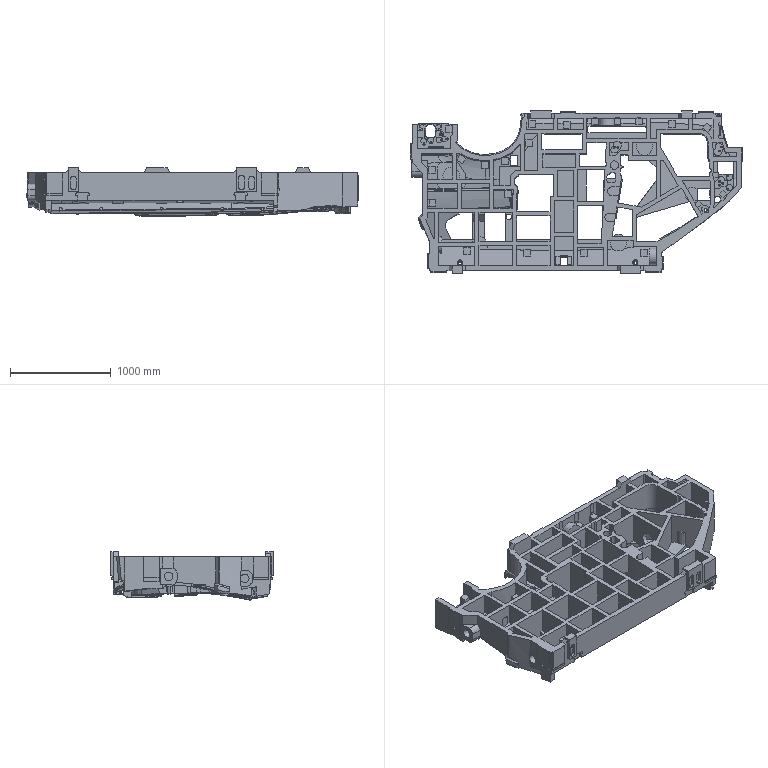Part | NX | features solid 2 | 1 solid | 2839 faces | box 3296 x 1615 x 481.661 mm | volume 562057370 mm3 | spline 1572 | plane 997 | cylinder 269 | sphere 1 | commonest cylinder face diameters 20 x37 40 x31 30 x28 52 x24 50 x19 165 x19